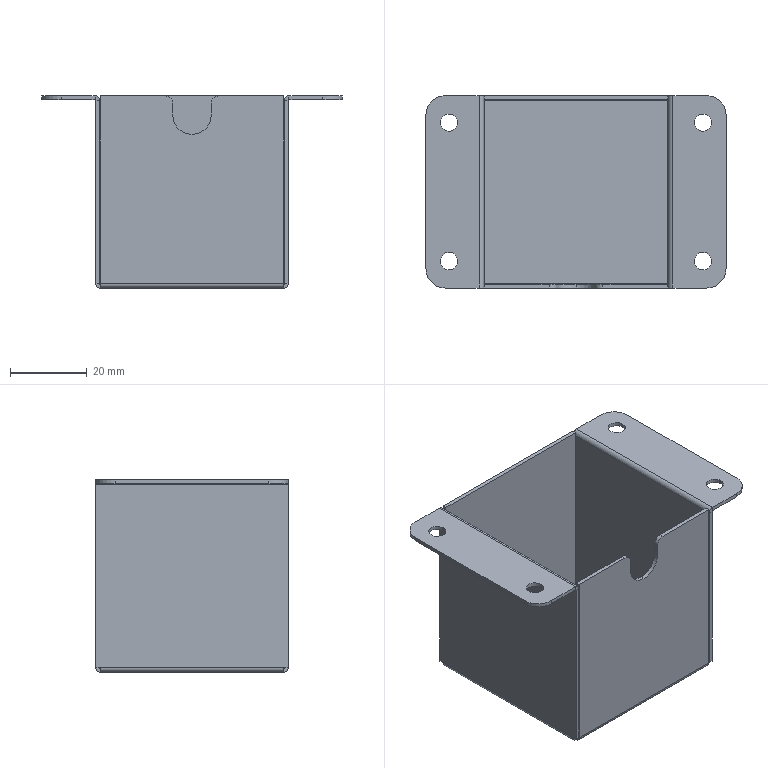Part | STEP file | Push button switch guard | 1 solid | 77 faces | box 78 x 50 x 50 mm | volume 13195 mm3 | plane 49 | cylinder 28 | commonest cylinder face diameters 4.5 x8 0.4 x6 2.4 x6 10 x6 4 x2